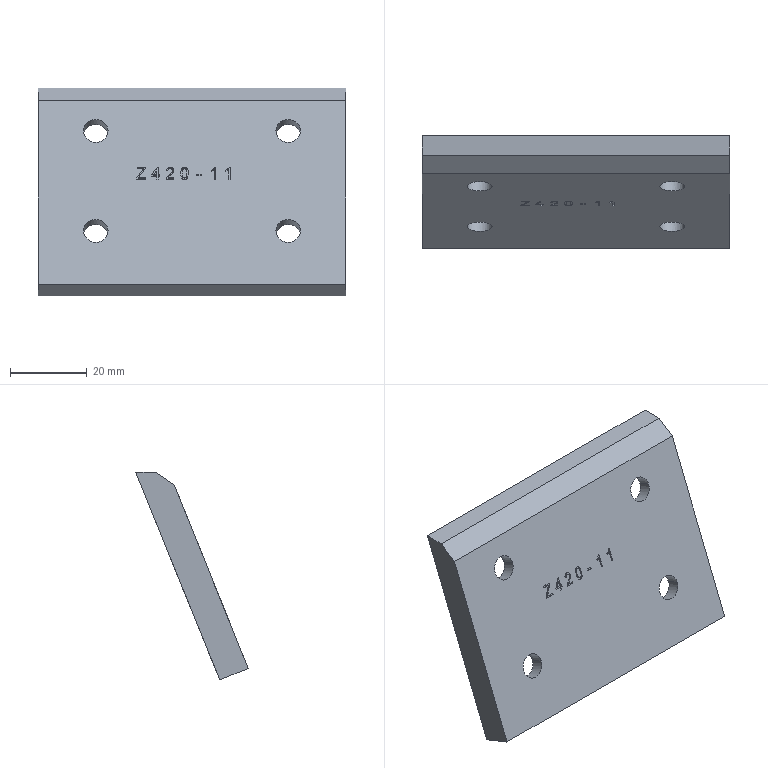Part | Creo | 1 solid | 122 faces | box 80 x 29.235 x 54 mm | volume 33545 mm3 | plane 53 | other 51 | cylinder 10 | cone 8 | commonest cylinder face diameters 6.4 x8 2.917 x1 45.999 x1